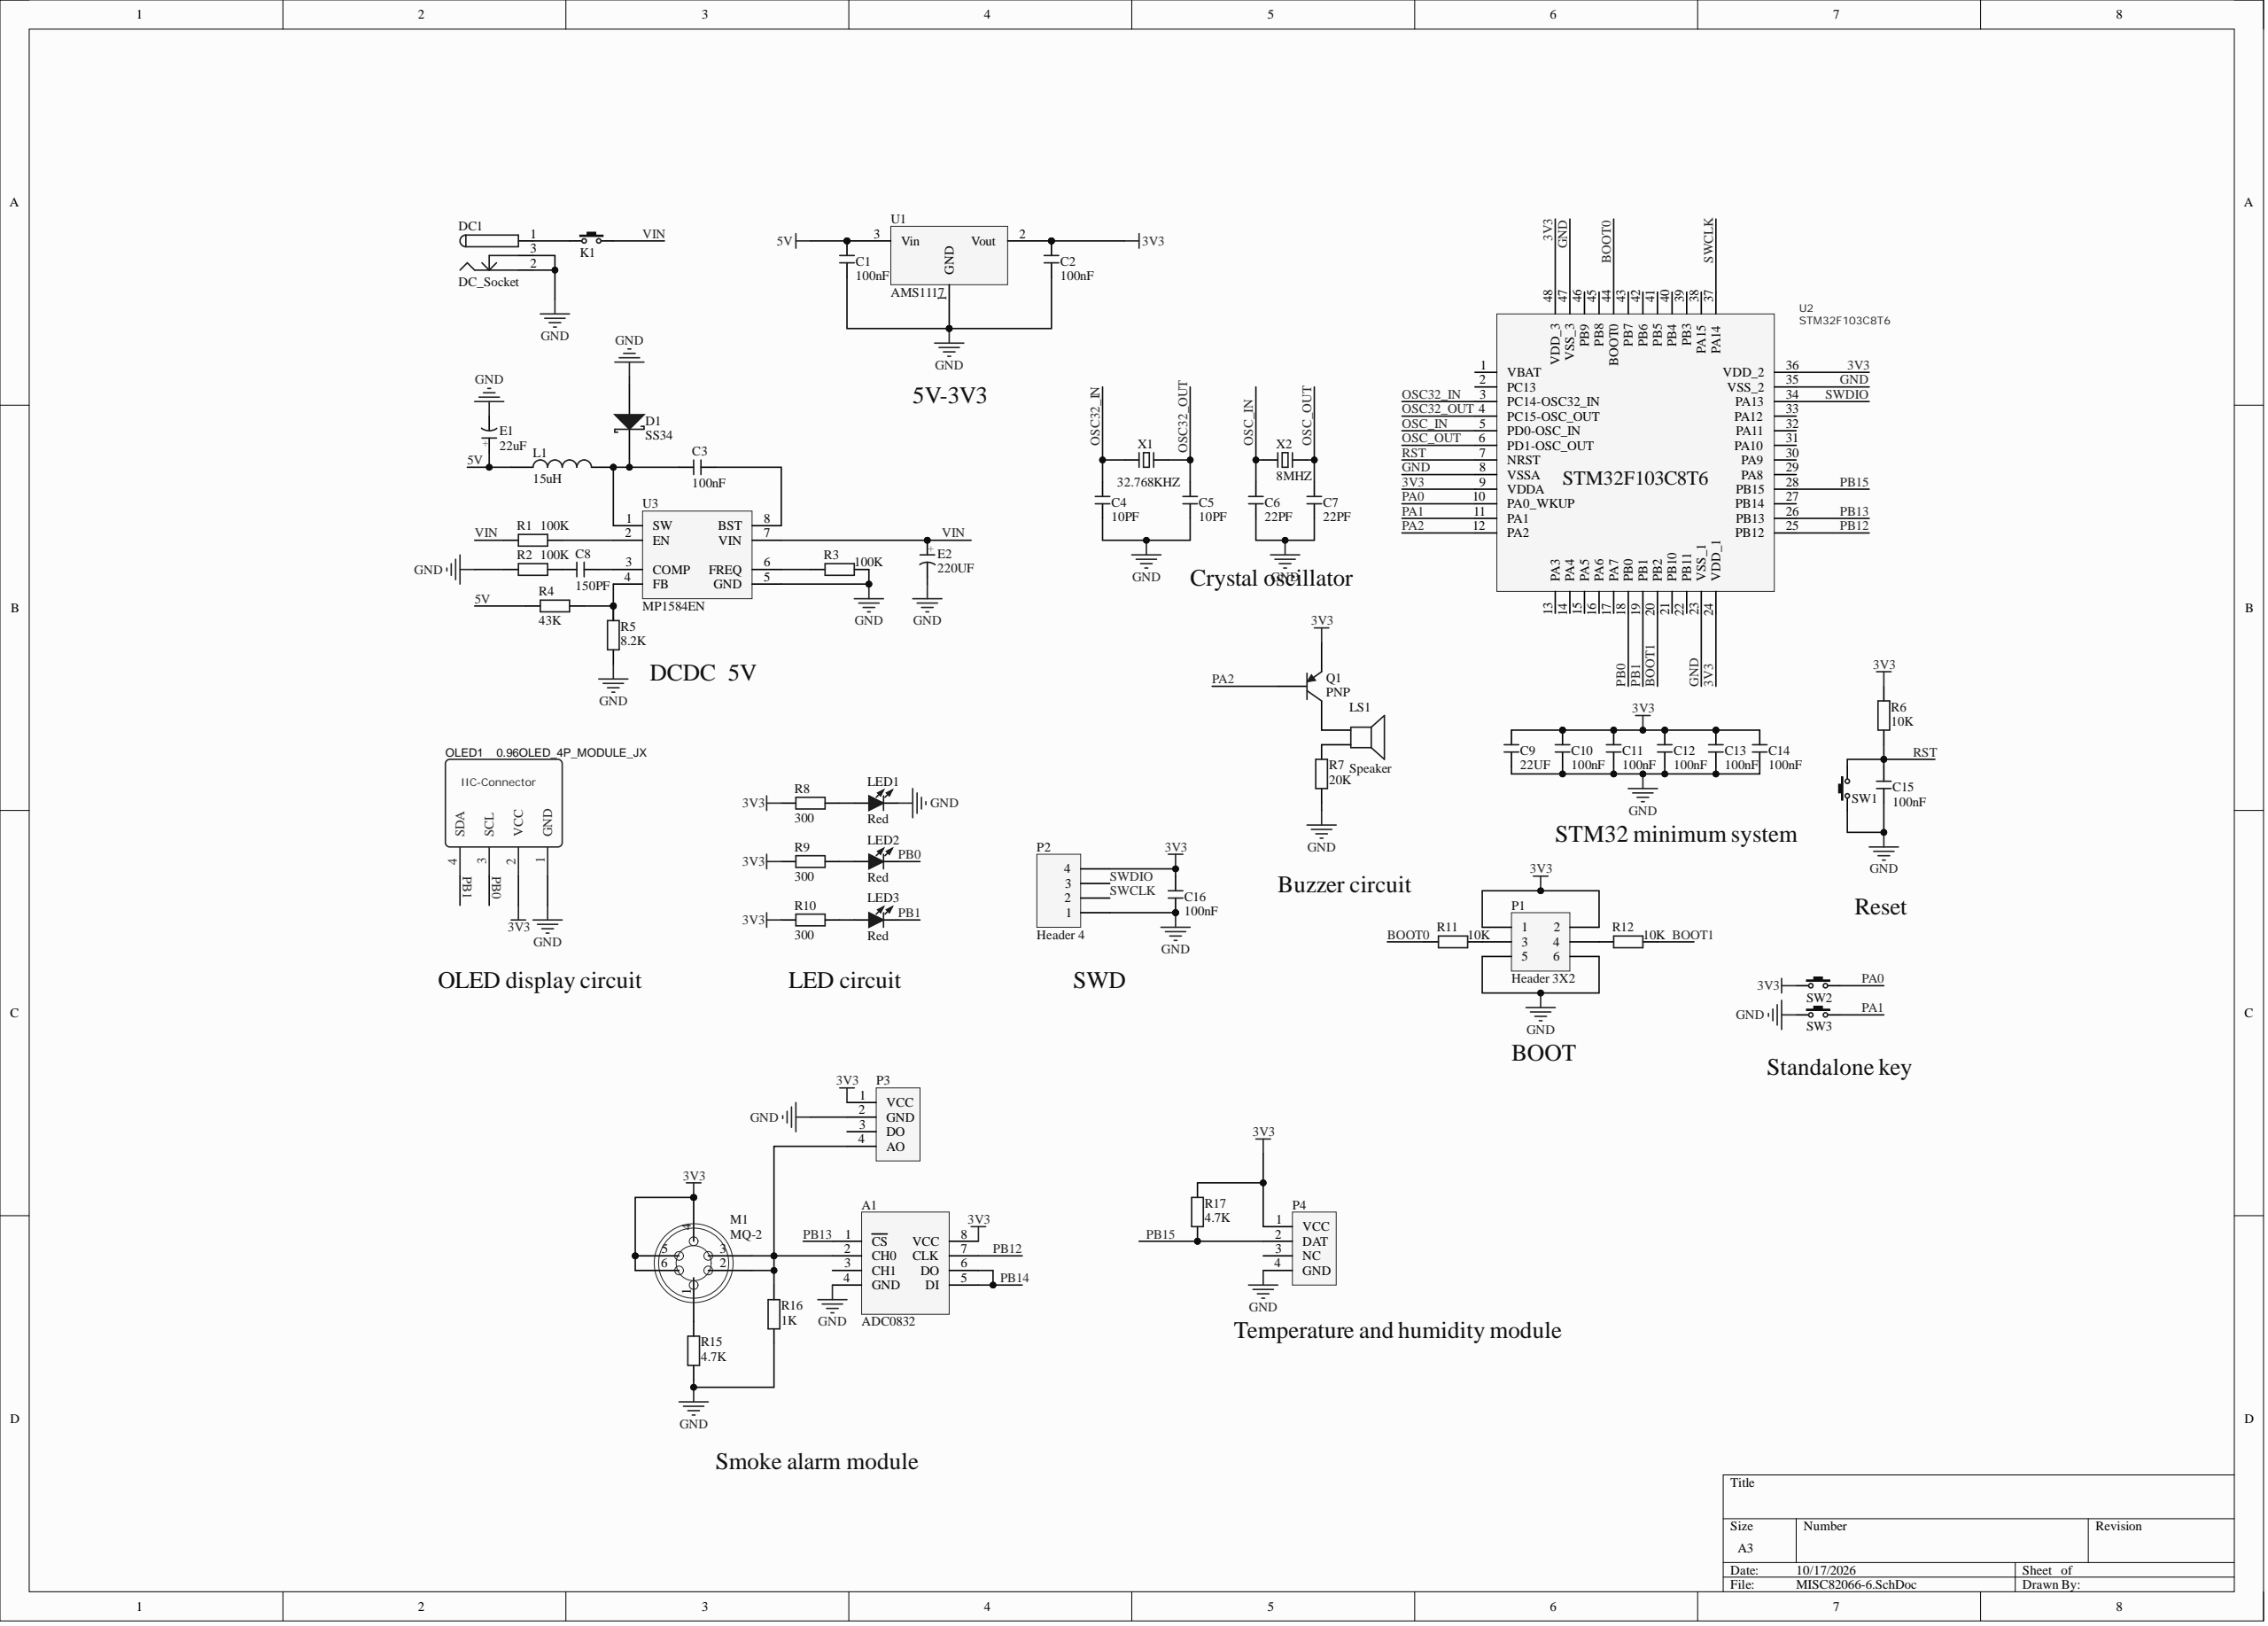Circuit board | Altium Designer | 57 parts | 39 nets
Bill of materials:
Comment,Description,Designator,Footprint,LibRef,Quantity
"ADC0832","","A1","DIP8","ADC0832","1"
"100nF","SMD capacitor","C1, C2, C3, C10, C11, C12, C13, C14, C15, C16","C 0805_L","C","10"
"10PF","SMD capacitor","C4, C5","C 0805_L","C","2"
"22PF","SMD capacitor","C6, C7","C 0805_L","C","2"
"150PF","SMD capacitor","C8","C 0805_L","C","1"
"22UF","SMD capacitor","C9","C 0805_L","C","1"
"SS34","Schottky diode","D1","SMC","SS34","1"
"DC_Socket","","DC1","DC-002","DC_Socket","1"
"22uF","SMD electrolytic capacitor","E1","CM A(3*5.4)","CE_SMD","1"
"220UF","SMD solid-state capacitor","E2","CT 5*6 - C","CS_SMD","1"
"6x6x5","Side-push through-hole 6x6 tact switch","K1","TSW DIP-6*6*6_V","TSW DIP-6x6_V","1"
"15uH","Low-power SMD inductor","L1","L 0805","L","1"
"Red","SMD LED","LED1, LED2, LED3","LED 0805G","LED-SMD","3"
"Speaker","Loudspeaker","LS1","PIN2","Speaker","1"
"MQ-2","Gas sensor","M1","MQ-2","MQ-2","1"
"0.96OLED_4P_MODULE_JX","","OLED1","0.96OLED_4P","0.96OLED_4P_MODULE_JX","1"
"Header 3X2","Header, 3-Pin, Dual row","P1","HDR2X3","Header 3X2","1"
"Header 4","Header, 4-Pin","P2, P3, P4","HDR1X4","Header 4","3"
"PNP","PNP Bipolar Transistor","Q1","SOT-23B_N","PNP","1"
"100K","SMD resistor","R1, R2, R3","R 0805_L","R","3"
"43K","SMD resistor","R4","R 0805_L","R","1"
"8.2K","SMD resistor","R5","R 0805_L","R","1"
"10K","SMD resistor","R6, R11, R12","R 0805_L","R","3"
"20K","SMD resistor","R7","R 0805_L","R","1"
"300","SMD resistor","R8, R9, R10","R 0805_L","R","3"
"4.7K","SMD resistor","R15, R17","R 0805_L","R","2"
"1K","SMD resistor","R16","R 0805_L","R","1"
"3x6x5","3x6 tact switch","SW1, SW2, SW3","TSW SMD-3*6*2.5","TSW 3x6","3"
"AMS1117","Three-terminal regulator IC","U1","SOT223","AMS1117","1"
"STM32F103C8T6","","U2","LQFP48 7X7","STM32F103C8T6","1"
"MP1584EN","","U3","MP1548EN","MP1584EN","1"
"32.768KHZ","2-pin passive crystal oscillator","X1","OSC HC-49S","XTAL-2P","1"
"8MHZ","2-pin passive crystal oscillator","X2","OSC HC-49S","XTAL-2P","1"
Netlist (Protel format):
[
A1
DIP8
ADC0832



]
[
C1
C 0805_L
100nF



]
[
C2
C 0805_L
100nF



]
[
C3
C 0805_L
100nF



]
[
C4
C 0805_L
10PF



]
[
C5
C 0805_L
10PF



]
[
C6
C 0805_L
22PF



]
[
C7
C 0805_L
22PF



]
[
C8
C 0805_L
150PF



]
[
C9
C 0805_L
22UF



]
[
C10
C 0805_L
100nF



]
[
C11
C 0805_L
100nF



]
[
C12
C 0805_L
100nF



]
[
C13
C 0805_L
100nF



]
[
C14
C 0805_L
100nF



]
[
C15
C 0805_L
100nF



]
[
C16
C 0805_L
100nF



]
[
D1
SMC
SS34



]
[
DC1
DC-002
DC_Socket



]
[
E1
CM A(3*5.4)
22uF



]
[
E2
CT 5*6 - C
220UF



]
[
K1
TSW DIP-6*6*6_V
6x6x5



]
[
L1
L 0805
15uH



]
[
LED1
LED 0805G
Red



]
[
LED2
LED 0805G
Red



]
[
LED3
LED 0805G
Red



]
[
LS1
PIN2
Speaker



]
[
M1
MQ-2
MQ-2



]
[
OLED1
0.96OLED_4P
0.96OLED_4P_MODULE_JX



]
[
P1
HDR2X3
Header 3X2



]
[
P2
HDR1X4
Header 4



]
[
P3
HDR1X4
Header 4



]
[
P4
HDR1X4
Header 4



]
[
Q1
SOT-23B_N
PNP



]
[
R1
R 0805_L
100K



]
[
R2
R 0805_L
100K



]
[
R3
R 0805_L
100K



]
[
R4
R 0805_L
43K



]
[
R5
R 0805_L
8.2K



]
[
R6
R 0805_L
10K



]
[
R7
R 0805_L
20K



]
[
R8
R 0805_L
300



]
[
R9
R 0805_L
300



]
[
R10
R 0805_L
300



]
[
R11
R 0805_L
10K



]
[
R12
R 0805_L
10K



]
[
R15
R 0805_L
4.7K



]
[
R16
R 0805_L
1K



]
[
R17
R 0805_L
4.7K



]
[
SW1
TSW SMD-3*6*2.5
3x6x5



]
[
SW2
TSW SMD-3*6*2.5
3x6x5



]
[
SW3
TSW SMD-3*6*2.5
3x6x5



]
[
U1
SOT223
AMS1117



]
[
U2
LQFP48 7X7
STM32F103C8T6



]
[
U3
MP1548EN
MP1584EN



]
[
X1
OSC HC-49S
32.768KHZ



]
[
X2
OSC HC-49S
8MHZ



]
(
VIN
E2-1
K1-2
R1-1
U3-7
)
(
SWDIO
P2-3
U2-34
)
(
SWCLK
P2-2
U2-37
)
(
RST
C15-2
R6-2
SW1-2
U2-7
)
(
PB15
P4-2
R17-2
U2-28
)
(
PB14
A1-5
A1-6
)
(
PB13
A1-1
U2-26
)
(
PB12
A1-7
U2-25
)
(
PB1
LED3-2
OLED1-4
U2-19
)
(
PB0
LED2-2
OLED1-3
U2-18
)
(
PA2
Q1-2
U2-12
)
(
PA1
SW3-2
U2-11
)
(
PA0
SW2-2
U2-10
)
(
OSC_OUT
C7-2
U2-6
X2-2
)
(
OSC_IN
C6-2
U2-5
X2-1
)
(
OSC32_OUT
C5-2
U2-4
X1-2
)
(
OSC32_IN
C4-2
U2-3
X1-1
)
(
NetR4_1
R4-1
R5-2
U3-4
)
(
NetR3_2
R3-2
U3-6
)
(
NetR1_2
R1-2
U3-2
)
(
NetP1_4
P1-4
R12-2
)
(
NetP1_3
P1-3
R11-1
)
(
NetM1_1
M1-1
R15-1
)
(
NetLS1_2
LS1-2
R7-1
)
(
NetLS1_1
LS1-1
Q1-1
)
(
NetLED3_1
LED3-1
R10-1
)
(
NetLED2_1
LED2-1
R9-1
)
(
NetLED1_1
LED1-1
R8-1
)
(
NetDC1_1
DC1-1
K1-1
)
(
NetC8_2
C8-2
U3-3
)
(
NetC8_1
C8-1
R2-2
)
(
NetC3_2
C3-2
U3-8
)
(
NetC3_1
C3-1
D1-2
L1-2
U3-1
)
(
NetA1_2
A1-2
M1-2
M1-3
P3-4
R16-1
)
(
GND
A1-4
C1-1
C2-1
C4-1
C5-1
C6-1
C7-1
C9-1
C10-1
C11-1
C12-1
C13-1
C14-1
C15-1
C16-1
D1-1
DC1-2
DC1-3
E1-2
E2-2
LED1-2
OLED1-1
P1-5
P1-6
P2-1
P3-2
P4-4
R2-1
R3-1
R5-1
R7-2
R15-2
R16-2
SW1-1
SW3-1
U1-1
U2-8
U2-23
U2-35
U2-47
U3-5
)
(
BOOT1
R12-1
U2-20
)
(
BOOT0
R11-2
U2-44
)
(
5V
C1-2
E1-1
L1-1
R4-2
U1-3
)
(
3V3
A1-8
C2-2
C9-2
C10-2
C11-2
C12-2
C13-2
C14-2
C16-2
M1-4
M1-5
M1-6
OLED1-2
P1-1
P1-2
P2-4
P3-1
P4-1
Q1-3
R6-1
R8-2
R9-2
R10-2
R17-1
SW2-1
U1-2
U2-9
U2-24
U2-36
U2-48
)